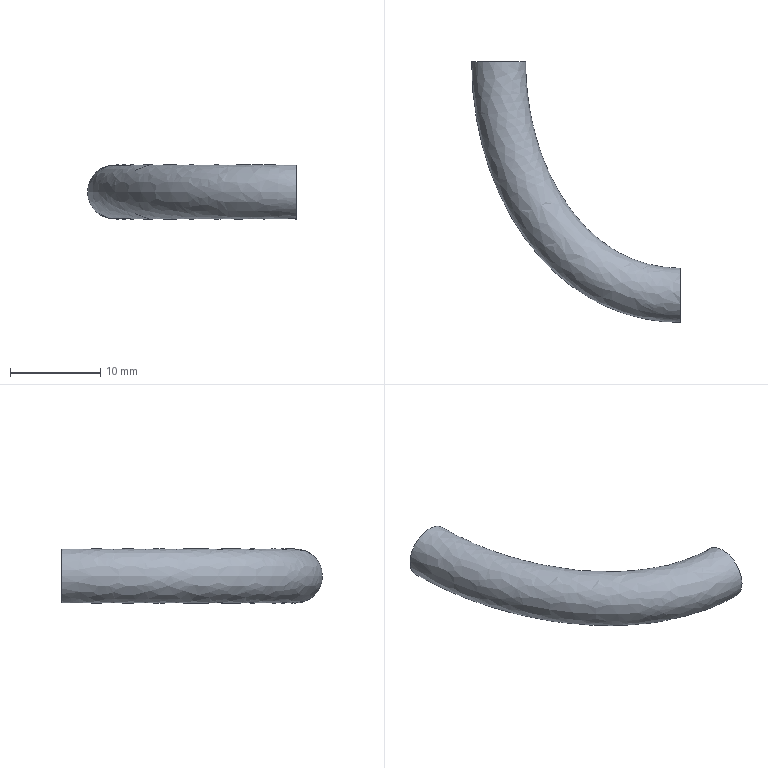Part | NX | features solid 2 | 1 solid | 4 faces | box 23.133 x 28.889 x 6 mm | volume 572.071 mm3 | plane 2 | spline 2